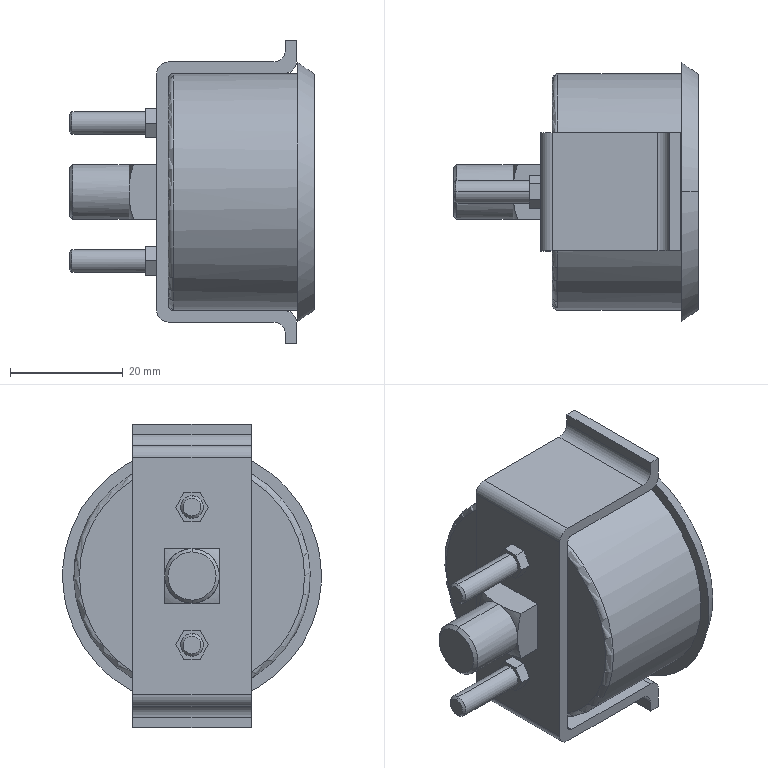Part | SolidWorks | features BaseBody 1 | 1 solid | 73 faces | box 43.5 x 46 x 54 mm | volume 41092 mm3 | plane 41 | cylinder 18 | cone 8 | torus 6 | commonest cylinder face diameters 4 x10 2 x2 9.728 x2 37.8 x2 42 x2